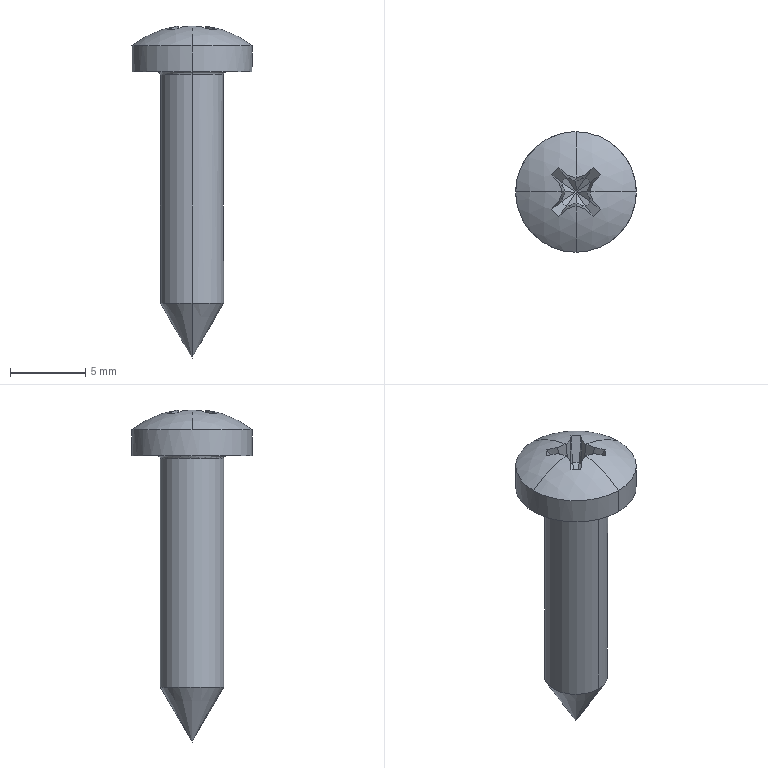Part | STEP file | 410151501000_ST4.2×19 | 1 solid | 45 faces | box 8 x 8 x 22.035 mm | volume 343.522 mm3 | plane 25 | spline 8 | cylinder 4 | sphere 4 | torus 2 | cone 2 | commonest cylinder face diameters 4.2 x2 8 x2